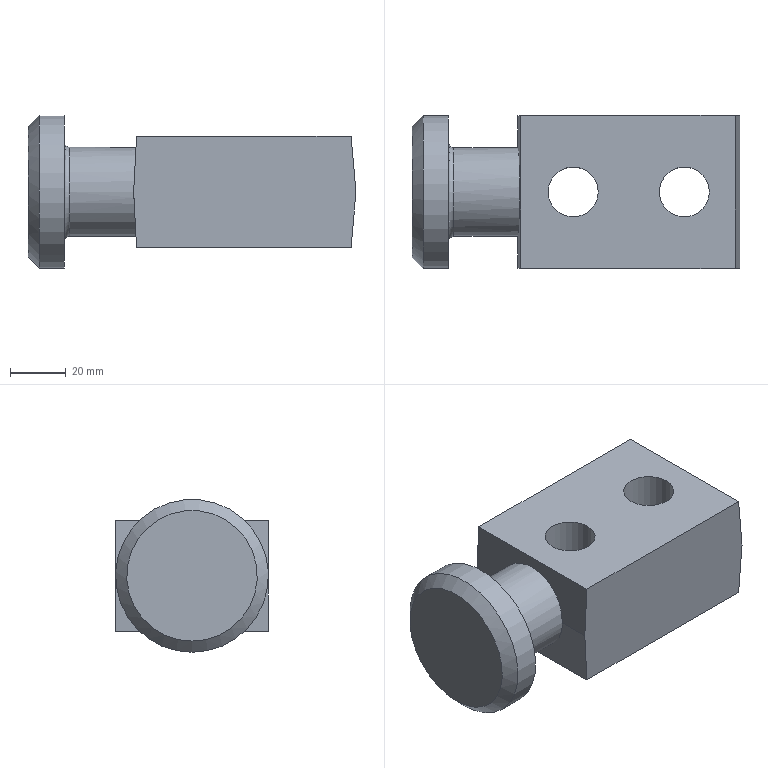Part | STEP file | CHP10_id1814_x_t | 1 solid | 88 faces | box 118 x 55 x 55 mm | volume 202286 mm3 | plane 41 | other 41 | cylinder 4 | torus 1 | cone 1 | commonest cylinder face diameters 18 x2 32 x1 55 x1